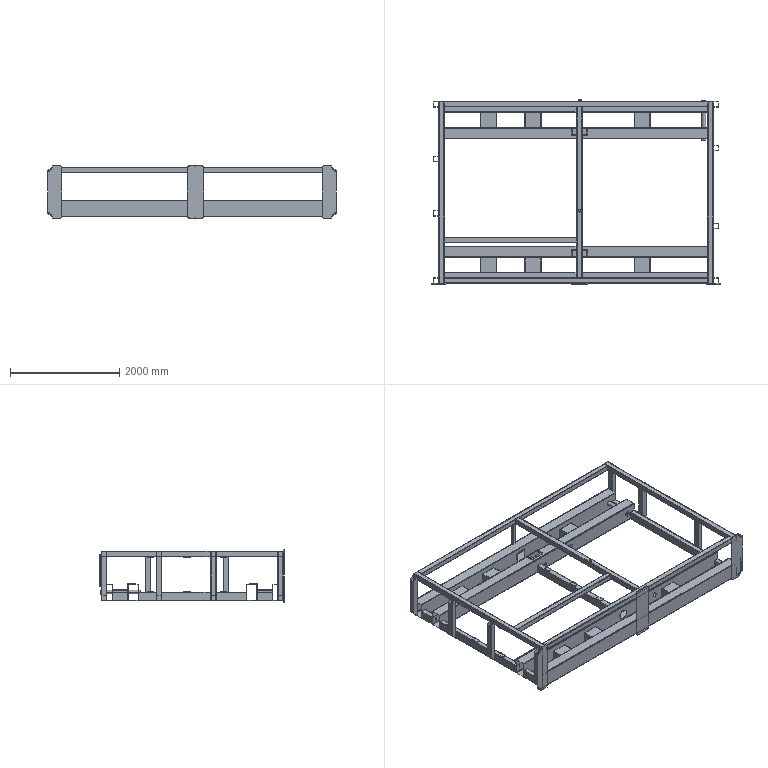Part | SolidWorks | features BaseBody 30, ICE 19, Chamfer 2, EdgeFlange 1, FlatPattern 1, LPattern 1, MirrorSolid 1, MoveFace 1, SMBaseFlange 1, SheetMetal 1 | 52 solids | 1043 faces | box 5290 x 3374 x 970 mm | volume 176959507 mm3 | cylinder 542 | plane 501 | commonest cylinder face diameters 6.8 x144 16 x100 8 x93 10 x89 20 x40 10.3 x24